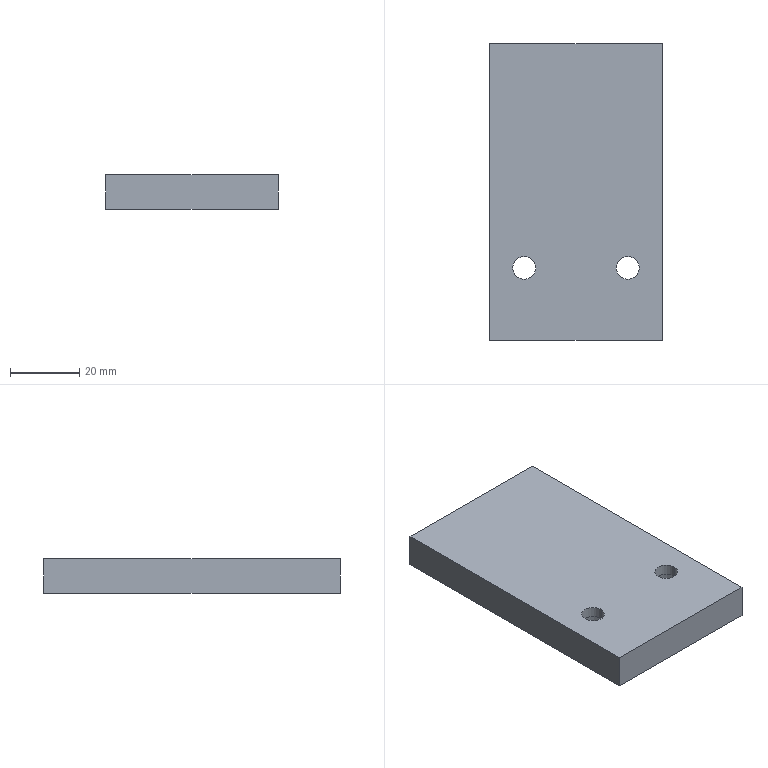Part | SolidWorks | features BaseBody 1 | 1 solid | 16 faces | box 50 x 86 x 10 mm | volume 41489 mm3 | cylinder 8 | plane 8 | commonest cylinder face diameters 6.6 x4 11 x4
STEP:
#1=CARTESIAN_POINT('',(1498.3,441.,-230.));
#2=VERTEX_POINT('',#1);
#3=CARTESIAN_POINT('',(1491.7,441.,-230.));
#4=VERTEX_POINT('',#3);
#5=CARTESIAN_POINT('',(1495.,441.,-230.));
#6=DIRECTION('',(0.,0.,-1.));
#7=DIRECTION('',(-1.,0.,0.));
#8=AXIS2_PLACEMENT_3D('',#5,#6,#7);
#9=CIRCLE('',#8,3.3);
#10=EDGE_CURVE('',#2,#4,#9,.T.);
#11=ORIENTED_EDGE('',*,*,#10,.F.);
#12=CARTESIAN_POINT('',(1498.3,441.,-233.2));
#13=VERTEX_POINT('',#12);
#14=CARTESIAN_POINT('',(1498.3,441.,-240.));
#15=DIRECTION('',(0.,0.,-1.));
#16=VECTOR('',#15,1000.);
#17=LINE('',#14,#16);
#18=EDGE_CURVE('',#2,#13,#17,.T.);
#19=ORIENTED_EDGE('',*,*,#18,.T.);
#20=CARTESIAN_POINT('',(1491.7,441.,-233.2));
#21=VERTEX_POINT('',#20);
#22=CARTESIAN_POINT('',(1495.,441.,-233.2));
#23=DIRECTION('',(0.,0.,-1.));
#24=DIRECTION('',(-1.,0.,0.));
#25=AXIS2_PLACEMENT_3D('',#22,#23,#24);
#26=CIRCLE('',#25,3.3);
#27=EDGE_CURVE('',#13,#21,#26,.T.);
#28=ORIENTED_EDGE('',*,*,#27,.T.);
#29=CARTESIAN_POINT('',(1491.7,441.,-240.));
#30=DIRECTION('',(0.,0.,-1.));
#31=VECTOR('',#30,1000.);
#32=LINE('',#29,#31);
#33=EDGE_CURVE('',#4,#21,#32,.T.);
#34=ORIENTED_EDGE('',*,*,#33,.F.);
#35=EDGE_LOOP('',(#11,#19,#28,#34));
#36=FACE_OUTER_BOUND('',#35,.T.);
#37=CARTESIAN_POINT('',(1495.,441.,-240.));
#38=DIRECTION('',(0.,0.,-1.));
#39=DIRECTION('',(-1.,0.,0.));
#40=AXIS2_PLACEMENT_3D('',#37,#38,#39);
#41=CYLINDRICAL_SURFACE('',#40,3.3);
#42=ADVANCED_FACE('',(#36),#41,.F.);
#43=CARTESIAN_POINT('',(1500.5,441.,-233.2));
#44=VERTEX_POINT('',#43);
#45=CARTESIAN_POINT('',(1489.5,441.,-233.2));
#46=VERTEX_POINT('',#45);
#47=CARTESIAN_POINT('',(1495.,441.,-233.2));
#48=DIRECTION('',(0.,0.,-1.));
#49=DIRECTION('',(-1.,0.,0.));
#50=AXIS2_PLACEMENT_3D('',#47,#48,#49);
#51=CIRCLE('',#50,5.5);
#52=EDGE_CURVE('',#44,#46,#51,.T.);
#53=ORIENTED_EDGE('',*,*,#52,.F.);
#54=CARTESIAN_POINT('',(1500.5,441.,-240.));
#55=VERTEX_POINT('',#54);
#56=CARTESIAN_POINT('',(1500.5,441.,-240.));
#57=DIRECTION('',(0.,0.,-1.));
#58=VECTOR('',#57,1000.);
#59=LINE('',#56,#58);
#60=EDGE_CURVE('',#44,#55,#59,.T.);
#61=ORIENTED_EDGE('',*,*,#60,.T.);
#62=CARTESIAN_POINT('',(1489.5,441.,-240.));
#63=VERTEX_POINT('',#62);
#64=CARTESIAN_POINT('',(1495.,441.,-240.));
#65=DIRECTION('',(0.,0.,-1.));
#66=DIRECTION('',(-1.,0.,0.));
#67=AXIS2_PLACEMENT_3D('',#64,#65,#66);
#68=CIRCLE('',#67,5.5);
#69=EDGE_CURVE('',#55,#63,#68,.T.);
#70=ORIENTED_EDGE('',*,*,#69,.T.);
#71=CARTESIAN_POINT('',(1489.5,441.,-240.));
#72=DIRECTION('',(0.,0.,-1.));
#73=VECTOR('',#72,1000.);
#74=LINE('',#71,#73);
#75=EDGE_CURVE('',#46,#63,#74,.T.);
#76=ORIENTED_EDGE('',*,*,#75,.F.);
#77=EDGE_LOOP('',(#53,#61,#70,#76));
#78=FACE_OUTER_BOUND('',#77,.T.);
#79=CARTESIAN_POINT('',(1495.,441.,-240.));
#80=DIRECTION('',(0.,0.,-1.));
#81=DIRECTION('',(-1.,0.,0.));
#82=AXIS2_PLACEMENT_3D('',#79,#80,#81);
#83=CYLINDRICAL_SURFACE('',#82,5.5);
#84=ADVANCED_FACE('',(#78),#83,.F.);
#85=CARTESIAN_POINT('',(1468.3,441.,-230.));
#86=VERTEX_POINT('',#85);
#87=CARTESIAN_POINT('',(1461.7,441.,-230.));
#88=VERTEX_POINT('',#87);
#89=CARTESIAN_POINT('',(1465.,441.,-230.));
#90=DIRECTION('',(0.,0.,-1.));
#91=DIRECTION('',(-1.,0.,0.));
#92=AXIS2_PLACEMENT_3D('',#89,#90,#91);
#93=CIRCLE('',#92,3.3);
#94=EDGE_CURVE('',#86,#88,#93,.T.);
#95=ORIENTED_EDGE('',*,*,#94,.F.);
#96=CARTESIAN_POINT('',(1468.3,441.,-233.2));
#97=VERTEX_POINT('',#96);
#98=CARTESIAN_POINT('',(1468.3,441.,-240.));
#99=DIRECTION('',(0.,0.,-1.));
#100=VECTOR('',#99,1000.);
#101=LINE('',#98,#100);
#102=EDGE_CURVE('',#86,#97,#101,.T.);
#103=ORIENTED_EDGE('',*,*,#102,.T.);
#104=CARTESIAN_POINT('',(1461.7,441.,-233.2));
#105=VERTEX_POINT('',#104);
#106=CARTESIAN_POINT('',(1465.,441.,-233.2));
#107=DIRECTION('',(0.,0.,-1.));
#108=DIRECTION('',(-1.,0.,0.));
#109=AXIS2_PLACEMENT_3D('',#106,#107,#108);
#110=CIRCLE('',#109,3.3);
#111=EDGE_CURVE('',#97,#105,#110,.T.);
#112=ORIENTED_EDGE('',*,*,#111,.T.);
#113=CARTESIAN_POINT('',(1461.7,441.,-240.));
#114=DIRECTION('',(0.,0.,-1.));
#115=VECTOR('',#114,1000.);
#116=LINE('',#113,#115);
#117=EDGE_CURVE('',#88,#105,#116,.T.);
#118=ORIENTED_EDGE('',*,*,#117,.F.);
#119=EDGE_LOOP('',(#95,#103,#112,#118));
#120=FACE_OUTER_BOUND('',#119,.T.);
#121=CARTESIAN_POINT('',(1465.,441.,-240.));
#122=DIRECTION('',(0.,0.,-1.));
#123=DIRECTION('',(-1.,0.,0.));
#124=AXIS2_PLACEMENT_3D('',#121,#122,#123);
#125=CYLINDRICAL_SURFACE('',#124,3.3);
#126=ADVANCED_FACE('',(#120),#125,.F.);
#127=CARTESIAN_POINT('',(1470.5,441.,-233.2));
#128=VERTEX_POINT('',#127);
#129=CARTESIAN_POINT('',(1459.5,441.,-233.2));
#130=VERTEX_POINT('',#129);
#131=CARTESIAN_POINT('',(1465.,441.,-233.2));
#132=DIRECTION('',(0.,0.,-1.));
#133=DIRECTION('',(-1.,0.,0.));
#134=AXIS2_PLACEMENT_3D('',#131,#132,#133);
#135=CIRCLE('',#134,5.5);
#136=EDGE_CURVE('',#128,#130,#135,.T.);
#137=ORIENTED_EDGE('',*,*,#136,.F.);
#138=CARTESIAN_POINT('',(1470.5,441.,-240.));
#139=VERTEX_POINT('',#138);
#140=CARTESIAN_POINT('',(1470.5,441.,-240.));
#141=DIRECTION('',(0.,0.,-1.));
#142=VECTOR('',#141,1000.);
#143=LINE('',#140,#142);
#144=EDGE_CURVE('',#128,#139,#143,.T.);
#145=ORIENTED_EDGE('',*,*,#144,.T.);
#146=CARTESIAN_POINT('',(1459.5,441.,-240.));
#147=VERTEX_POINT('',#146);
#148=CARTESIAN_POINT('',(1465.,441.,-240.));
#149=DIRECTION('',(0.,0.,-1.));
#150=DIRECTION('',(-1.,0.,0.));
#151=AXIS2_PLACEMENT_3D('',#148,#149,#150);
#152=CIRCLE('',#151,5.5);
#153=EDGE_CURVE('',#139,#147,#152,.T.);
#154=ORIENTED_EDGE('',*,*,#153,.T.);
#155=CARTESIAN_POINT('',(1459.5,441.,-240.));
#156=DIRECTION('',(0.,0.,-1.));
#157=VECTOR('',#156,1000.);
#158=LINE('',#155,#157);
#159=EDGE_CURVE('',#130,#147,#158,.T.);
#160=ORIENTED_EDGE('',*,*,#159,.F.);
#161=EDGE_LOOP('',(#137,#145,#154,#160));
#162=FACE_OUTER_BOUND('',#161,.T.);
#163=CARTESIAN_POINT('',(1465.,441.,-240.));
#164=DIRECTION('',(0.,0.,-1.));
#165=DIRECTION('',(-1.,0.,0.));
#166=AXIS2_PLACEMENT_3D('',#163,#164,#165);
#167=CYLINDRICAL_SURFACE('',#166,5.5);
#168=ADVANCED_FACE('',(#162),#167,.F.);
#169=CARTESIAN_POINT('',(1505.,420.,-240.));
#170=VERTEX_POINT('',#169);
#171=CARTESIAN_POINT('',(1505.,420.,-230.));
#172=VERTEX_POINT('',#171);
#173=CARTESIAN_POINT('',(1505.,420.,-230.));
#174=DIRECTION('',(0.,0.,1.));
#175=VECTOR('',#174,1000.);
#176=LINE('',#173,#175);
#177=EDGE_CURVE('',#170,#172,#176,.T.);
#178=ORIENTED_EDGE('',*,*,#177,.T.);
#179=CARTESIAN_POINT('',(1455.,420.,-230.));
#180=VERTEX_POINT('',#179);
#181=CARTESIAN_POINT('',(0.,420.,-230.));
#182=DIRECTION('',(1.,0.,0.));
#183=VECTOR('',#182,1000.);
#184=LINE('',#181,#183);
#185=EDGE_CURVE('',#180,#172,#184,.T.);
#186=ORIENTED_EDGE('',*,*,#185,.F.);
#187=CARTESIAN_POINT('',(1455.,420.,-240.));
#188=VERTEX_POINT('',#187);
#189=CARTESIAN_POINT('',(1455.,420.,-230.));
#190=DIRECTION('',(0.,0.,-1.));
#191=VECTOR('',#190,1000.);
#192=LINE('',#189,#191);
#193=EDGE_CURVE('',#180,#188,#192,.T.);
#194=ORIENTED_EDGE('',*,*,#193,.T.);
#195=CARTESIAN_POINT('',(0.,420.,-240.));
#196=DIRECTION('',(1.,0.,0.));
#197=VECTOR('',#196,1000.);
#198=LINE('',#195,#197);
#199=EDGE_CURVE('',#188,#170,#198,.T.);
#200=ORIENTED_EDGE('',*,*,#199,.T.);
#201=EDGE_LOOP('',(#178,#186,#194,#200));
#202=FACE_OUTER_BOUND('',#201,.T.);
#203=CARTESIAN_POINT('',(1402.456,420.,-220.));
#204=DIRECTION('',(0.,1.,0.));
#205=DIRECTION('',(1.,0.,0.));
#206=AXIS2_PLACEMENT_3D('',#203,#204,#205);
#207=PLANE('',#206);
#208=ADVANCED_FACE('',(#202),#207,.F.);
#209=CARTESIAN_POINT('',(1505.,506.,-240.));
#210=VERTEX_POINT('',#209);
#211=CARTESIAN_POINT('',(1455.,506.,-240.));
#212=VERTEX_POINT('',#211);
#213=CARTESIAN_POINT('',(1505.,506.,-240.));
#214=DIRECTION('',(-1.,0.,0.));
#215=VECTOR('',#214,1000.);
#216=LINE('',#213,#215);
#217=EDGE_CURVE('',#210,#212,#216,.T.);
#218=ORIENTED_EDGE('',*,*,#217,.T.);
#219=CARTESIAN_POINT('',(1455.,506.,-230.));
#220=VERTEX_POINT('',#219);
#221=CARTESIAN_POINT('',(1455.,506.,-230.));
#222=DIRECTION('',(0.,0.,1.));
#223=VECTOR('',#222,1000.);
#224=LINE('',#221,#223);
#225=EDGE_CURVE('',#212,#220,#224,.T.);
#226=ORIENTED_EDGE('',*,*,#225,.T.);
#227=CARTESIAN_POINT('',(1505.,506.,-230.));
#228=VERTEX_POINT('',#227);
#229=CARTESIAN_POINT('',(1505.,506.,-230.));
#230=DIRECTION('',(-1.,0.,0.));
#231=VECTOR('',#230,1000.);
#232=LINE('',#229,#231);
#233=EDGE_CURVE('',#228,#220,#232,.T.);
#234=ORIENTED_EDGE('',*,*,#233,.F.);
#235=CARTESIAN_POINT('',(1505.,506.,-230.));
#236=DIRECTION('',(0.,0.,1.));
#237=VECTOR('',#236,1000.);
#238=LINE('',#235,#237);
#239=EDGE_CURVE('',#210,#228,#238,.T.);
#240=ORIENTED_EDGE('',*,*,#239,.F.);
#241=EDGE_LOOP('',(#218,#226,#234,#240));
#242=FACE_OUTER_BOUND('',#241,.T.);
#243=CARTESIAN_POINT('',(-9973.619,506.,-234.));
#244=DIRECTION('',(0.,-1.,0.));
#245=DIRECTION('',(0.,0.,-1.));
#246=AXIS2_PLACEMENT_3D('',#243,#244,#245);
#247=PLANE('',#246);
#248=ADVANCED_FACE('',(#242),#247,.F.);
#249=CARTESIAN_POINT('',(1495.,441.,-233.2));
#250=DIRECTION('',(0.,0.,-1.));
#251=DIRECTION('',(-1.,0.,0.));
#252=AXIS2_PLACEMENT_3D('',#249,#250,#251);
#253=CIRCLE('',#252,3.3);
#254=EDGE_CURVE('',#21,#13,#253,.T.);
#255=ORIENTED_EDGE('',*,*,#254,.F.);
#256=ORIENTED_EDGE('',*,*,#27,.F.);
#257=EDGE_LOOP('',(#255,#256));
#258=FACE_BOUND('',#257,.T.);
#259=CARTESIAN_POINT('',(1495.,441.,-233.2));
#260=DIRECTION('',(0.,0.,-1.));
#261=DIRECTION('',(-1.,0.,0.));
#262=AXIS2_PLACEMENT_3D('',#259,#260,#261);
#263=CIRCLE('',#262,5.5);
#264=EDGE_CURVE('',#46,#44,#263,.T.);
#265=ORIENTED_EDGE('',*,*,#264,.T.);
#266=ORIENTED_EDGE('',*,*,#52,.T.);
#267=EDGE_LOOP('',(#265,#266));
#268=FACE_OUTER_BOUND('',#267,.T.);
#269=CARTESIAN_POINT('',(1498.3,441.,-233.2));
#270=DIRECTION('',(0.,0.,1.));
#271=DIRECTION('',(1.,0.,0.));
#272=AXIS2_PLACEMENT_3D('',#269,#270,#271);
#273=PLANE('',#272);
#274=ADVANCED_FACE('',(#258,#268),#273,.F.);
#275=CARTESIAN_POINT('',(1465.,441.,-233.2));
#276=DIRECTION('',(0.,0.,-1.));
#277=DIRECTION('',(-1.,0.,0.));
#278=AXIS2_PLACEMENT_3D('',#275,#276,#277);
#279=CIRCLE('',#278,3.3);
#280=EDGE_CURVE('',#105,#97,#279,.T.);
#281=ORIENTED_EDGE('',*,*,#280,.F.);
#282=ORIENTED_EDGE('',*,*,#111,.F.);
#283=EDGE_LOOP('',(#281,#282));
#284=FACE_BOUND('',#283,.T.);
#285=CARTESIAN_POINT('',(1465.,441.,-233.2));
#286=DIRECTION('',(0.,0.,-1.));
#287=DIRECTION('',(-1.,0.,0.));
#288=AXIS2_PLACEMENT_3D('',#285,#286,#287);
#289=CIRCLE('',#288,5.5);
#290=EDGE_CURVE('',#130,#128,#289,.T.);
#291=ORIENTED_EDGE('',*,*,#290,.T.);
#292=ORIENTED_EDGE('',*,*,#136,.T.);
#293=EDGE_LOOP('',(#291,#292));
#294=FACE_OUTER_BOUND('',#293,.T.);
#295=CARTESIAN_POINT('',(1468.3,441.,-233.2));
#296=DIRECTION('',(0.,0.,1.));
#297=DIRECTION('',(1.,0.,0.));
#298=AXIS2_PLACEMENT_3D('',#295,#296,#297);
#299=PLANE('',#298);
#300=ADVANCED_FACE('',(#284,#294),#299,.F.);
#301=CARTESIAN_POINT('',(1495.,441.,-240.));
#302=DIRECTION('',(0.,0.,-1.));
#303=DIRECTION('',(-1.,0.,0.));
#304=AXIS2_PLACEMENT_3D('',#301,#302,#303);
#305=CIRCLE('',#304,5.5);
#306=EDGE_CURVE('',#63,#55,#305,.T.);
#307=ORIENTED_EDGE('',*,*,#306,.F.);
#308=ORIENTED_EDGE('',*,*,#69,.F.);
#309=EDGE_LOOP('',(#307,#308));
#310=FACE_BOUND('',#309,.T.);
#311=CARTESIAN_POINT('',(1465.,441.,-240.));
#312=DIRECTION('',(0.,0.,-1.));
#313=DIRECTION('',(-1.,0.,0.));
#314=AXIS2_PLACEMENT_3D('',#311,#312,#313);
#315=CIRCLE('',#314,5.5);
#316=EDGE_CURVE('',#147,#139,#315,.T.);
#317=ORIENTED_EDGE('',*,*,#316,.F.);
#318=ORIENTED_EDGE('',*,*,#153,.F.);
#319=EDGE_LOOP('',(#317,#318));
#320=FACE_BOUND('',#319,.T.);
#321=ORIENTED_EDGE('',*,*,#199,.F.);
#322=CARTESIAN_POINT('',(1455.,496.,-240.));
#323=DIRECTION('',(0.,1.,0.));
#324=VECTOR('',#323,1000.);
#325=LINE('',#322,#324);
#326=EDGE_CURVE('',#188,#212,#325,.T.);
#327=ORIENTED_EDGE('',*,*,#326,.T.);
#328=ORIENTED_EDGE('',*,*,#217,.F.);
#329=CARTESIAN_POINT('',(1505.,496.,-240.));
#330=DIRECTION('',(0.,-1.,0.));
#331=VECTOR('',#330,1000.);
#332=LINE('',#329,#331);
#333=EDGE_CURVE('',#210,#170,#332,.T.);
#334=ORIENTED_EDGE('',*,*,#333,.T.);
#335=EDGE_LOOP('',(#321,#327,#328,#334));
#336=FACE_OUTER_BOUND('',#335,.T.);
#337=CARTESIAN_POINT('',(0.,0.,-240.));
#338=DIRECTION('',(0.,0.,-1.));
#339=DIRECTION('',(0.,-1.,0.));
#340=AXIS2_PLACEMENT_3D('',#337,#338,#339);
#341=PLANE('',#340);
#342=ADVANCED_FACE('',(#310,#320,#336),#341,.T.);
#343=CARTESIAN_POINT('',(1495.,441.,-230.));
#344=DIRECTION('',(0.,0.,-1.));
#345=DIRECTION('',(-1.,0.,0.));
#346=AXIS2_PLACEMENT_3D('',#343,#344,#345);
#347=CIRCLE('',#346,3.3);
#348=EDGE_CURVE('',#4,#2,#347,.T.);
#349=ORIENTED_EDGE('',*,*,#348,.T.);
#350=ORIENTED_EDGE('',*,*,#10,.T.);
#351=EDGE_LOOP('',(#349,#350));
#352=FACE_BOUND('',#351,.T.);
#353=CARTESIAN_POINT('',(1465.,441.,-230.));
#354=DIRECTION('',(0.,0.,-1.));
#355=DIRECTION('',(-1.,0.,0.));
#356=AXIS2_PLACEMENT_3D('',#353,#354,#355);
#357=CIRCLE('',#356,3.3);
#358=EDGE_CURVE('',#88,#86,#357,.T.);
#359=ORIENTED_EDGE('',*,*,#358,.T.);
#360=ORIENTED_EDGE('',*,*,#94,.T.);
#361=EDGE_LOOP('',(#359,#360));
#362=FACE_BOUND('',#361,.T.);
#363=CARTESIAN_POINT('',(1455.,496.,-230.));
#364=DIRECTION('',(0.,1.,0.));
#365=VECTOR('',#364,1000.);
#366=LINE('',#363,#365);
#367=EDGE_CURVE('',#180,#220,#366,.T.);
#368=ORIENTED_EDGE('',*,*,#367,.F.);
#369=ORIENTED_EDGE('',*,*,#185,.T.);
#370=CARTESIAN_POINT('',(1505.,496.,-230.));
#371=DIRECTION('',(0.,-1.,0.));
#372=VECTOR('',#371,1000.);
#373=LINE('',#370,#372);
#374=EDGE_CURVE('',#228,#172,#373,.T.);
#375=ORIENTED_EDGE('',*,*,#374,.F.);
#376=ORIENTED_EDGE('',*,*,#233,.T.);
#377=EDGE_LOOP('',(#368,#369,#375,#376));
#378=FACE_OUTER_BOUND('',#377,.T.);
#379=CARTESIAN_POINT('',(0.,0.,-230.));
#380=DIRECTION('',(0.,0.,-1.));
#381=DIRECTION('',(0.,-1.,0.));
#382=AXIS2_PLACEMENT_3D('',#379,#380,#381);
#383=PLANE('',#382);
#384=ADVANCED_FACE('',(#352,#362,#378),#383,.F.);
#385=ORIENTED_EDGE('',*,*,#193,.F.);
#386=ORIENTED_EDGE('',*,*,#367,.T.);
#387=ORIENTED_EDGE('',*,*,#225,.F.);
#388=ORIENTED_EDGE('',*,*,#326,.F.);
#389=EDGE_LOOP('',(#385,#386,#387,#388));
#390=FACE_OUTER_BOUND('',#389,.T.);
#391=CARTESIAN_POINT('',(1455.,496.,-230.));
#392=DIRECTION('',(-1.,0.,0.));
#393=DIRECTION('',(0.,0.,1.));
#394=AXIS2_PLACEMENT_3D('',#391,#392,#393);
#395=PLANE('',#394);
#396=ADVANCED_FACE('',(#390),#395,.T.);
#397=ORIENTED_EDGE('',*,*,#177,.F.);
#398=ORIENTED_EDGE('',*,*,#333,.F.);
#399=ORIENTED_EDGE('',*,*,#239,.T.);
#400=ORIENTED_EDGE('',*,*,#374,.T.);
#401=EDGE_LOOP('',(#397,#398,#399,#400));
#402=FACE_OUTER_BOUND('',#401,.T.);
#403=CARTESIAN_POINT('',(1505.,496.,-230.));
#404=DIRECTION('',(1.,0.,0.));
#405=DIRECTION('',(0.,1.,0.));
#406=AXIS2_PLACEMENT_3D('',#403,#404,#405);
#407=PLANE('',#406);
#408=ADVANCED_FACE('',(#402),#407,.T.);
#409=ORIENTED_EDGE('',*,*,#144,.F.);
#410=ORIENTED_EDGE('',*,*,#290,.F.);
#411=ORIENTED_EDGE('',*,*,#159,.T.);
#412=ORIENTED_EDGE('',*,*,#316,.T.);
#413=EDGE_LOOP('',(#409,#410,#411,#412));
#414=FACE_OUTER_BOUND('',#413,.T.);
#415=CARTESIAN_POINT('',(1465.,441.,-240.));
#416=DIRECTION('',(0.,0.,-1.));
#417=DIRECTION('',(-1.,0.,0.));
#418=AXIS2_PLACEMENT_3D('',#415,#416,#417);
#419=CYLINDRICAL_SURFACE('',#418,5.5);
#420=ADVANCED_FACE('',(#414),#419,.F.);
#421=ORIENTED_EDGE('',*,*,#102,.F.);
#422=ORIENTED_EDGE('',*,*,#358,.F.);
#423=ORIENTED_EDGE('',*,*,#117,.T.);
#424=ORIENTED_EDGE('',*,*,#280,.T.);
#425=EDGE_LOOP('',(#421,#422,#423,#424));
#426=FACE_OUTER_BOUND('',#425,.T.);
#427=CARTESIAN_POINT('',(1465.,441.,-240.));
#428=DIRECTION('',(0.,0.,-1.));
#429=DIRECTION('',(-1.,0.,0.));
#430=AXIS2_PLACEMENT_3D('',#427,#428,#429);
#431=CYLINDRICAL_SURFACE('',#430,3.3);
#432=ADVANCED_FACE('',(#426),#431,.F.);
#433=ORIENTED_EDGE('',*,*,#60,.F.);
#434=ORIENTED_EDGE('',*,*,#264,.F.);
#435=ORIENTED_EDGE('',*,*,#75,.T.);
#436=ORIENTED_EDGE('',*,*,#306,.T.);
#437=EDGE_LOOP('',(#433,#434,#435,#436));
#438=FACE_OUTER_BOUND('',#437,.T.);
#439=CARTESIAN_POINT('',(1495.,441.,-240.));
#440=DIRECTION('',(0.,0.,-1.));
#441=DIRECTION('',(-1.,0.,0.));
#442=AXIS2_PLACEMENT_3D('',#439,#440,#441);
#443=CYLINDRICAL_SURFACE('',#442,5.5);
#444=ADVANCED_FACE('',(#438),#443,.F.);
#445=ORIENTED_EDGE('',*,*,#18,.F.);
#446=ORIENTED_EDGE('',*,*,#348,.F.);
#447=ORIENTED_EDGE('',*,*,#33,.T.);
#448=ORIENTED_EDGE('',*,*,#254,.T.);
#449=EDGE_LOOP('',(#445,#446,#447,#448));
#450=FACE_OUTER_BOUND('',#449,.T.);
#451=CARTESIAN_POINT('',(1495.,441.,-240.));
#452=DIRECTION('',(0.,0.,-1.));
#453=DIRECTION('',(-1.,0.,0.));
#454=AXIS2_PLACEMENT_3D('',#451,#452,#453);
#455=CYLINDRICAL_SURFACE('',#454,3.3);
#456=ADVANCED_FACE('',(#450),#455,.F.);
#457=CLOSED_SHELL('',(#42,#84,#126,#168,#208,#248,#274,#300,#342,#384,#396,#408,#420,#432,#444,#456));
#458=MANIFOLD_SOLID_BREP('',#457);
#459=CARTESIAN_POINT('',(0.,0.,0.));
#460=DIRECTION('',(0.,0.,1.));
#461=DIRECTION('',(1.,0.,0.));
#462=AXIS2_PLACEMENT_3D('',#459,#460,#461);
#463=(LENGTH_UNIT()NAMED_UNIT(*)SI_UNIT(.MILLI.,.METRE.));
#464=UNCERTAINTY_MEASURE_WITH_UNIT(LENGTH_MEASURE(0.00001),#463,'','');
#465=(NAMED_UNIT(*)PLANE_ANGLE_UNIT()SI_UNIT($,.RADIAN.));
#466=(NAMED_UNIT(*)SI_UNIT($,.STERADIAN.)SOLID_ANGLE_UNIT());
#467=(GEOMETRIC_REPRESENTATION_CONTEXT(3)GLOBAL_UNCERTAINTY_ASSIGNED_CONTEXT((#464))GLOBAL_UNIT_ASSIGNED_CONTEXT((#463,#465,#466))REPRESENTATION_CONTEXT('',''));
#468=ADVANCED_BREP_SHAPE_REPRESENTATION('',(#458,#462),#467);